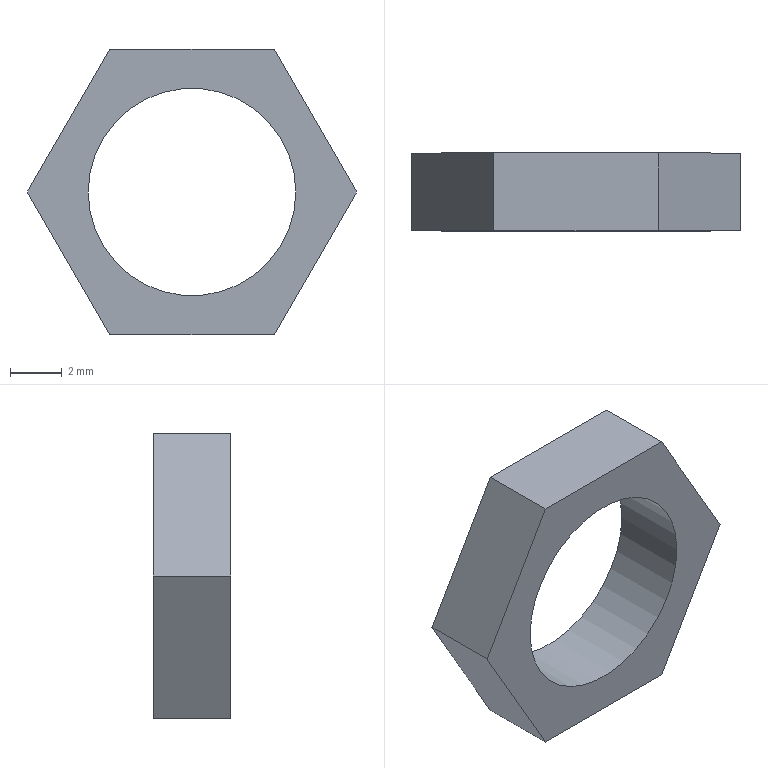Part | STEP file | 1-28.7 | 1 solid | 9 faces | box 12.702 x 3 x 11 mm | volume 163.571 mm3 | plane 8 | cylinder 1 | commonest cylinder face diameters 8 x1
STEP:
#1=CARTESIAN_POINT('',(0.,0.,0.));
#2=DIRECTION('',(0.,0.,1.));
#3=DIRECTION('',(1.,0.,0.));
#4=AXIS2_PLACEMENT_3D('',#1,#2,#3);
#5=CARTESIAN_POINT('',(6.351,0.,0.));
#6=VERTEX_POINT('',#5);
#7=CARTESIAN_POINT('',(3.175,0.,5.5));
#8=VERTEX_POINT('',#7);
#9=CARTESIAN_POINT('',(6.351,0.,0.));
#10=DIRECTION('',(-0.5,0.,0.866));
#11=VECTOR('',#10,1.);
#12=LINE('',#9,#11);
#13=CARTESIAN_POINT('',(0.,0.,0.8509));
#14=DIRECTION('',(0.,-1.,0.));
#15=DIRECTION('',(1.,0.,0.));
#16=AXIS2_PLACEMENT_3D('',#13,#14,#15);
#17=PLANE('',#16);
#18=CARTESIAN_POINT('',(6.351,-0.8509));
#19=DIRECTION('',(-0.5,0.866));
#20=VECTOR('',#19,1.);
#21=LINE('',#18,#20);
#22=(GEOMETRIC_REPRESENTATION_CONTEXT(2)PARAMETRIC_REPRESENTATION_CONTEXT()REPRESENTATION_CONTEXT('',''));
#23=DEFINITIONAL_REPRESENTATION('',(#21),#22);
#24=PCURVE('',#17,#23);
#25=CARTESIAN_POINT('',(4.763,1.5,2.75));
#26=DIRECTION('',(-0.866,0.,-0.5));
#27=DIRECTION('',(-0.5,0.,0.866));
#28=AXIS2_PLACEMENT_3D('',#25,#26,#27);
#29=PLANE('',#28);
#30=CARTESIAN_POINT('',(-3.175,-1.5));
#31=DIRECTION('',(1.,0.));
#32=VECTOR('',#31,1.);
#33=LINE('',#30,#32);
#34=(GEOMETRIC_REPRESENTATION_CONTEXT(2)PARAMETRIC_REPRESENTATION_CONTEXT()REPRESENTATION_CONTEXT('',''));
#35=DEFINITIONAL_REPRESENTATION('',(#33),#34);
#36=PCURVE('',#29,#35);
#37=SURFACE_CURVE('',#12,(#24,#36),.PCURVE_S1.);
#38=EDGE_CURVE('',#6,#8,#37,.T.);
#39=ORIENTED_EDGE('',*,*,#38,.T.);
#40=CARTESIAN_POINT('',(-3.175,0.,5.5));
#41=VERTEX_POINT('',#40);
#42=CARTESIAN_POINT('',(3.175,0.,5.5));
#43=DIRECTION('',(-1.,0.,0.));
#44=VECTOR('',#43,1.);
#45=LINE('',#42,#44);
#46=CARTESIAN_POINT('',(3.175,4.649));
#47=DIRECTION('',(-1.,0.));
#48=VECTOR('',#47,1.);
#49=LINE('',#46,#48);
#50=(GEOMETRIC_REPRESENTATION_CONTEXT(2)PARAMETRIC_REPRESENTATION_CONTEXT()REPRESENTATION_CONTEXT('',''));
#51=DEFINITIONAL_REPRESENTATION('',(#49),#50);
#52=PCURVE('',#17,#51);
#53=CARTESIAN_POINT('',(0.,1.5,5.5));
#54=DIRECTION('',(0.,0.,-1.));
#55=DIRECTION('',(-1.,0.,0.));
#56=AXIS2_PLACEMENT_3D('',#53,#54,#55);
#57=PLANE('',#56);
#58=CARTESIAN_POINT('',(-3.175,-1.5));
#59=DIRECTION('',(1.,0.));
#60=VECTOR('',#59,1.);
#61=LINE('',#58,#60);
#62=(GEOMETRIC_REPRESENTATION_CONTEXT(2)PARAMETRIC_REPRESENTATION_CONTEXT()REPRESENTATION_CONTEXT('',''));
#63=DEFINITIONAL_REPRESENTATION('',(#61),#62);
#64=PCURVE('',#57,#63);
#65=SURFACE_CURVE('',#45,(#52,#64),.PCURVE_S1.);
#66=EDGE_CURVE('',#8,#41,#65,.T.);
#67=ORIENTED_EDGE('',*,*,#66,.T.);
#68=CARTESIAN_POINT('',(-6.351,0.,0.));
#69=VERTEX_POINT('',#68);
#70=CARTESIAN_POINT('',(-3.175,0.,5.5));
#71=DIRECTION('',(-0.5,0.,-0.866));
#72=VECTOR('',#71,1.);
#73=LINE('',#70,#72);
#74=CARTESIAN_POINT('',(-3.175,4.649));
#75=DIRECTION('',(-0.5,-0.866));
#76=VECTOR('',#75,1.);
#77=LINE('',#74,#76);
#78=(GEOMETRIC_REPRESENTATION_CONTEXT(2)PARAMETRIC_REPRESENTATION_CONTEXT()REPRESENTATION_CONTEXT('',''));
#79=DEFINITIONAL_REPRESENTATION('',(#77),#78);
#80=PCURVE('',#17,#79);
#81=CARTESIAN_POINT('',(-4.763,1.5,2.75));
#82=DIRECTION('',(0.866,0.,-0.5));
#83=DIRECTION('',(-0.5,0.,-0.866));
#84=AXIS2_PLACEMENT_3D('',#81,#82,#83);
#85=PLANE('',#84);
#86=CARTESIAN_POINT('',(-3.175,-1.5));
#87=DIRECTION('',(1.,0.));
#88=VECTOR('',#87,1.);
#89=LINE('',#86,#88);
#90=(GEOMETRIC_REPRESENTATION_CONTEXT(2)PARAMETRIC_REPRESENTATION_CONTEXT()REPRESENTATION_CONTEXT('',''));
#91=DEFINITIONAL_REPRESENTATION('',(#89),#90);
#92=PCURVE('',#85,#91);
#93=SURFACE_CURVE('',#73,(#80,#92),.PCURVE_S1.);
#94=EDGE_CURVE('',#41,#69,#93,.T.);
#95=ORIENTED_EDGE('',*,*,#94,.T.);
#96=CARTESIAN_POINT('',(-3.175,0.,-5.5));
#97=VERTEX_POINT('',#96);
#98=CARTESIAN_POINT('',(-6.351,0.,0.));
#99=DIRECTION('',(0.5,0.,-0.866));
#100=VECTOR('',#99,1.);
#101=LINE('',#98,#100);
#102=CARTESIAN_POINT('',(-6.351,-0.8509));
#103=DIRECTION('',(0.5,-0.866));
#104=VECTOR('',#103,1.);
#105=LINE('',#102,#104);
#106=(GEOMETRIC_REPRESENTATION_CONTEXT(2)PARAMETRIC_REPRESENTATION_CONTEXT()REPRESENTATION_CONTEXT('',''));
#107=DEFINITIONAL_REPRESENTATION('',(#105),#106);
#108=PCURVE('',#17,#107);
#109=CARTESIAN_POINT('',(-4.763,1.5,-2.75));
#110=DIRECTION('',(0.866,0.,0.5));
#111=DIRECTION('',(0.5,0.,-0.866));
#112=AXIS2_PLACEMENT_3D('',#109,#110,#111);
#113=PLANE('',#112);
#114=CARTESIAN_POINT('',(-3.175,-1.5));
#115=DIRECTION('',(1.,0.));
#116=VECTOR('',#115,1.);
#117=LINE('',#114,#116);
#118=(GEOMETRIC_REPRESENTATION_CONTEXT(2)PARAMETRIC_REPRESENTATION_CONTEXT()REPRESENTATION_CONTEXT('',''));
#119=DEFINITIONAL_REPRESENTATION('',(#117),#118);
#120=PCURVE('',#113,#119);
#121=SURFACE_CURVE('',#101,(#108,#120),.PCURVE_S1.);
#122=EDGE_CURVE('',#69,#97,#121,.T.);
#123=ORIENTED_EDGE('',*,*,#122,.T.);
#124=CARTESIAN_POINT('',(3.175,0.,-5.5));
#125=VERTEX_POINT('',#124);
#126=CARTESIAN_POINT('',(-3.175,0.,-5.5));
#127=DIRECTION('',(1.,0.,0.));
#128=VECTOR('',#127,1.);
#129=LINE('',#126,#128);
#130=CARTESIAN_POINT('',(-3.175,-6.351));
#131=DIRECTION('',(1.,0.));
#132=VECTOR('',#131,1.);
#133=LINE('',#130,#132);
#134=(GEOMETRIC_REPRESENTATION_CONTEXT(2)PARAMETRIC_REPRESENTATION_CONTEXT()REPRESENTATION_CONTEXT('',''));
#135=DEFINITIONAL_REPRESENTATION('',(#133),#134);
#136=PCURVE('',#17,#135);
#137=CARTESIAN_POINT('',(0.,1.5,-5.5));
#138=DIRECTION('',(0.,0.,1.));
#139=DIRECTION('',(1.,0.,0.));
#140=AXIS2_PLACEMENT_3D('',#137,#138,#139);
#141=PLANE('',#140);
#142=CARTESIAN_POINT('',(-3.175,-1.5));
#143=DIRECTION('',(1.,0.));
#144=VECTOR('',#143,1.);
#145=LINE('',#142,#144);
#146=(GEOMETRIC_REPRESENTATION_CONTEXT(2)PARAMETRIC_REPRESENTATION_CONTEXT()REPRESENTATION_CONTEXT('',''));
#147=DEFINITIONAL_REPRESENTATION('',(#145),#146);
#148=PCURVE('',#141,#147);
#149=SURFACE_CURVE('',#129,(#136,#148),.PCURVE_S1.);
#150=EDGE_CURVE('',#97,#125,#149,.T.);
#151=ORIENTED_EDGE('',*,*,#150,.T.);
#152=CARTESIAN_POINT('',(3.175,0.,-5.5));
#153=DIRECTION('',(0.5,0.,0.866));
#154=VECTOR('',#153,1.);
#155=LINE('',#152,#154);
#156=CARTESIAN_POINT('',(3.175,-6.351));
#157=DIRECTION('',(0.5,0.866));
#158=VECTOR('',#157,1.);
#159=LINE('',#156,#158);
#160=(GEOMETRIC_REPRESENTATION_CONTEXT(2)PARAMETRIC_REPRESENTATION_CONTEXT()REPRESENTATION_CONTEXT('',''));
#161=DEFINITIONAL_REPRESENTATION('',(#159),#160);
#162=PCURVE('',#17,#161);
#163=CARTESIAN_POINT('',(4.763,1.5,-2.75));
#164=DIRECTION('',(-0.866,0.,0.5));
#165=DIRECTION('',(0.5,0.,0.866));
#166=AXIS2_PLACEMENT_3D('',#163,#164,#165);
#167=PLANE('',#166);
#168=CARTESIAN_POINT('',(-3.175,-1.5));
#169=DIRECTION('',(1.,0.));
#170=VECTOR('',#169,1.);
#171=LINE('',#168,#170);
#172=(GEOMETRIC_REPRESENTATION_CONTEXT(2)PARAMETRIC_REPRESENTATION_CONTEXT()REPRESENTATION_CONTEXT('',''));
#173=DEFINITIONAL_REPRESENTATION('',(#171),#172);
#174=PCURVE('',#167,#173);
#175=SURFACE_CURVE('',#155,(#162,#174),.PCURVE_S1.);
#176=EDGE_CURVE('',#125,#6,#175,.T.);
#177=ORIENTED_EDGE('',*,*,#176,.T.);
#178=EDGE_LOOP('',(#39,#67,#95,#123,#151,#177));
#179=FACE_BOUND('',#178,.T.);
#180=CARTESIAN_POINT('',(4.,0.,0.));
#181=VERTEX_POINT('',#180);
#182=CARTESIAN_POINT('',(0.,0.,0.));
#183=DIRECTION('',(0.,1.,0.));
#184=DIRECTION('',(1.,0.,0.));
#185=AXIS2_PLACEMENT_3D('',#182,#183,#184);
#186=CIRCLE('',#185,4.);
#187=CARTESIAN_POINT('',(4.,-0.8509));
#188=CARTESIAN_POINT('',(4.,-7.779));
#189=CARTESIAN_POINT('',(-2.,-4.315));
#190=CARTESIAN_POINT('',(-8.,-0.8509));
#191=CARTESIAN_POINT('',(-2.,2.613));
#192=CARTESIAN_POINT('',(4.,6.077));
#193=CARTESIAN_POINT('',(4.,-0.8509));
#194=(BOUNDED_CURVE()B_SPLINE_CURVE(2,(#187,#188,#189,#190,#191,#192,#193),.UNSPECIFIED.,.T.,.F.)B_SPLINE_CURVE_WITH_KNOTS((1,2,2,2,2,1),(-2.094,0.,2.094,4.189,6.283,8.378),.UNSPECIFIED.)CURVE()GEOMETRIC_REPRESENTATION_ITEM()RATIONAL_B_SPLINE_CURVE((1.,0.5,1.,0.5,1.,0.5,1.))REPRESENTATION_ITEM(''));
#195=(GEOMETRIC_REPRESENTATION_CONTEXT(2)PARAMETRIC_REPRESENTATION_CONTEXT()REPRESENTATION_CONTEXT('',''));
#196=DEFINITIONAL_REPRESENTATION('',(#194),#195);
#197=PCURVE('',#17,#196);
#198=CARTESIAN_POINT('',(0.,0.,0.));
#199=DIRECTION('',(0.,1.,0.));
#200=DIRECTION('',(1.,0.,0.));
#201=AXIS2_PLACEMENT_3D('',#198,#199,#200);
#202=CYLINDRICAL_SURFACE('',#201,4.);
#203=CARTESIAN_POINT('',(0.,0.));
#204=DIRECTION('',(1.,0.));
#205=VECTOR('',#204,1.);
#206=LINE('',#203,#205);
#207=(GEOMETRIC_REPRESENTATION_CONTEXT(2)PARAMETRIC_REPRESENTATION_CONTEXT()REPRESENTATION_CONTEXT('',''));
#208=DEFINITIONAL_REPRESENTATION('',(#206),#207);
#209=PCURVE('',#202,#208);
#210=SURFACE_CURVE('',#186,(#197,#209),.PCURVE_S1.);
#211=EDGE_CURVE('',#181,#181,#210,.T.);
#212=ORIENTED_EDGE('',*,*,#211,.T.);
#213=EDGE_LOOP('',(#212));
#214=FACE_BOUND('',#213,.T.);
#215=ADVANCED_FACE('',(#179,#214),#17,.T.);
#216=CARTESIAN_POINT('',(6.351,3.,0.));
#217=VERTEX_POINT('',#216);
#218=CARTESIAN_POINT('',(3.175,3.,5.5));
#219=VERTEX_POINT('',#218);
#220=CARTESIAN_POINT('',(6.351,3.,0.));
#221=DIRECTION('',(-0.5,0.,0.866));
#222=VECTOR('',#221,1.);
#223=LINE('',#220,#222);
#224=CARTESIAN_POINT('',(0.,3.,0.8509));
#225=DIRECTION('',(0.,-1.,0.));
#226=DIRECTION('',(1.,0.,0.));
#227=AXIS2_PLACEMENT_3D('',#224,#225,#226);
#228=PLANE('',#227);
#229=CARTESIAN_POINT('',(6.351,-0.8509));
#230=DIRECTION('',(-0.5,0.866));
#231=VECTOR('',#230,1.);
#232=LINE('',#229,#231);
#233=(GEOMETRIC_REPRESENTATION_CONTEXT(2)PARAMETRIC_REPRESENTATION_CONTEXT()REPRESENTATION_CONTEXT('',''));
#234=DEFINITIONAL_REPRESENTATION('',(#232),#233);
#235=PCURVE('',#228,#234);
#236=CARTESIAN_POINT('',(-3.175,1.5));
#237=DIRECTION('',(1.,0.));
#238=VECTOR('',#237,1.);
#239=LINE('',#236,#238);
#240=(GEOMETRIC_REPRESENTATION_CONTEXT(2)PARAMETRIC_REPRESENTATION_CONTEXT()REPRESENTATION_CONTEXT('',''));
#241=DEFINITIONAL_REPRESENTATION('',(#239),#240);
#242=PCURVE('',#29,#241);
#243=SURFACE_CURVE('',#223,(#235,#242),.PCURVE_S1.);
#244=EDGE_CURVE('',#217,#219,#243,.T.);
#245=ORIENTED_EDGE('',*,*,#244,.T.);
#246=CARTESIAN_POINT('',(-3.175,3.,5.5));
#247=VERTEX_POINT('',#246);
#248=CARTESIAN_POINT('',(3.175,3.,5.5));
#249=DIRECTION('',(-1.,0.,0.));
#250=VECTOR('',#249,1.);
#251=LINE('',#248,#250);
#252=CARTESIAN_POINT('',(3.175,4.649));
#253=DIRECTION('',(-1.,0.));
#254=VECTOR('',#253,1.);
#255=LINE('',#252,#254);
#256=(GEOMETRIC_REPRESENTATION_CONTEXT(2)PARAMETRIC_REPRESENTATION_CONTEXT()REPRESENTATION_CONTEXT('',''));
#257=DEFINITIONAL_REPRESENTATION('',(#255),#256);
#258=PCURVE('',#228,#257);
#259=CARTESIAN_POINT('',(-3.175,1.5));
#260=DIRECTION('',(1.,0.));
#261=VECTOR('',#260,1.);
#262=LINE('',#259,#261);
#263=(GEOMETRIC_REPRESENTATION_CONTEXT(2)PARAMETRIC_REPRESENTATION_CONTEXT()REPRESENTATION_CONTEXT('',''));
#264=DEFINITIONAL_REPRESENTATION('',(#262),#263);
#265=PCURVE('',#57,#264);
#266=SURFACE_CURVE('',#251,(#258,#265),.PCURVE_S1.);
#267=EDGE_CURVE('',#219,#247,#266,.T.);
#268=ORIENTED_EDGE('',*,*,#267,.T.);
#269=CARTESIAN_POINT('',(-6.351,3.,0.));
#270=VERTEX_POINT('',#269);
#271=CARTESIAN_POINT('',(-3.175,3.,5.5));
#272=DIRECTION('',(-0.5,0.,-0.866));
#273=VECTOR('',#272,1.);
#274=LINE('',#271,#273);
#275=CARTESIAN_POINT('',(-3.175,4.649));
#276=DIRECTION('',(-0.5,-0.866));
#277=VECTOR('',#276,1.);
#278=LINE('',#275,#277);
#279=(GEOMETRIC_REPRESENTATION_CONTEXT(2)PARAMETRIC_REPRESENTATION_CONTEXT()REPRESENTATION_CONTEXT('',''));
#280=DEFINITIONAL_REPRESENTATION('',(#278),#279);
#281=PCURVE('',#228,#280);
#282=CARTESIAN_POINT('',(-3.175,1.5));
#283=DIRECTION('',(1.,0.));
#284=VECTOR('',#283,1.);
#285=LINE('',#282,#284);
#286=(GEOMETRIC_REPRESENTATION_CONTEXT(2)PARAMETRIC_REPRESENTATION_CONTEXT()REPRESENTATION_CONTEXT('',''));
#287=DEFINITIONAL_REPRESENTATION('',(#285),#286);
#288=PCURVE('',#85,#287);
#289=SURFACE_CURVE('',#274,(#281,#288),.PCURVE_S1.);
#290=EDGE_CURVE('',#247,#270,#289,.T.);
#291=ORIENTED_EDGE('',*,*,#290,.T.);
#292=CARTESIAN_POINT('',(-3.175,3.,-5.5));
#293=VERTEX_POINT('',#292);
#294=CARTESIAN_POINT('',(-6.351,3.,0.));
#295=DIRECTION('',(0.5,0.,-0.866));
#296=VECTOR('',#295,1.);
#297=LINE('',#294,#296);
#298=CARTESIAN_POINT('',(-6.351,-0.8509));
#299=DIRECTION('',(0.5,-0.866));
#300=VECTOR('',#299,1.);
#301=LINE('',#298,#300);
#302=(GEOMETRIC_REPRESENTATION_CONTEXT(2)PARAMETRIC_REPRESENTATION_CONTEXT()REPRESENTATION_CONTEXT('',''));
#303=DEFINITIONAL_REPRESENTATION('',(#301),#302);
#304=PCURVE('',#228,#303);
#305=CARTESIAN_POINT('',(-3.175,1.5));
#306=DIRECTION('',(1.,0.));
#307=VECTOR('',#306,1.);
#308=LINE('',#305,#307);
#309=(GEOMETRIC_REPRESENTATION_CONTEXT(2)PARAMETRIC_REPRESENTATION_CONTEXT()REPRESENTATION_CONTEXT('',''));
#310=DEFINITIONAL_REPRESENTATION('',(#308),#309);
#311=PCURVE('',#113,#310);
#312=SURFACE_CURVE('',#297,(#304,#311),.PCURVE_S1.);
#313=EDGE_CURVE('',#270,#293,#312,.T.);
#314=ORIENTED_EDGE('',*,*,#313,.T.);
#315=CARTESIAN_POINT('',(3.175,3.,-5.5));
#316=VERTEX_POINT('',#315);
#317=CARTESIAN_POINT('',(-3.175,3.,-5.5));
#318=DIRECTION('',(1.,0.,0.));
#319=VECTOR('',#318,1.);
#320=LINE('',#317,#319);
#321=CARTESIAN_POINT('',(-3.175,-6.351));
#322=DIRECTION('',(1.,0.));
#323=VECTOR('',#322,1.);
#324=LINE('',#321,#323);
#325=(GEOMETRIC_REPRESENTATION_CONTEXT(2)PARAMETRIC_REPRESENTATION_CONTEXT()REPRESENTATION_CONTEXT('',''));
#326=DEFINITIONAL_REPRESENTATION('',(#324),#325);
#327=PCURVE('',#228,#326);
#328=CARTESIAN_POINT('',(-3.175,1.5));
#329=DIRECTION('',(1.,0.));
#330=VECTOR('',#329,1.);
#331=LINE('',#328,#330);
#332=(GEOMETRIC_REPRESENTATION_CONTEXT(2)PARAMETRIC_REPRESENTATION_CONTEXT()REPRESENTATION_CONTEXT('',''));
#333=DEFINITIONAL_REPRESENTATION('',(#331),#332);
#334=PCURVE('',#141,#333);
#335=SURFACE_CURVE('',#320,(#327,#334),.PCURVE_S1.);
#336=EDGE_CURVE('',#293,#316,#335,.T.);
#337=ORIENTED_EDGE('',*,*,#336,.T.);
#338=CARTESIAN_POINT('',(3.175,3.,-5.5));
#339=DIRECTION('',(0.5,0.,0.866));
#340=VECTOR('',#339,1.);
#341=LINE('',#338,#340);
#342=CARTESIAN_POINT('',(3.175,-6.351));
#343=DIRECTION('',(0.5,0.866));
#344=VECTOR('',#343,1.);
#345=LINE('',#342,#344);
#346=(GEOMETRIC_REPRESENTATION_CONTEXT(2)PARAMETRIC_REPRESENTATION_CONTEXT()REPRESENTATION_CONTEXT('',''));
#347=DEFINITIONAL_REPRESENTATION('',(#345),#346);
#348=PCURVE('',#228,#347);
#349=CARTESIAN_POINT('',(-3.175,1.5));
#350=DIRECTION('',(1.,0.));
#351=VECTOR('',#350,1.);
#352=LINE('',#349,#351);
#353=(GEOMETRIC_REPRESENTATION_CONTEXT(2)PARAMETRIC_REPRESENTATION_CONTEXT()REPRESENTATION_CONTEXT('',''));
#354=DEFINITIONAL_REPRESENTATION('',(#352),#353);
#355=PCURVE('',#167,#354);
#356=SURFACE_CURVE('',#341,(#348,#355),.PCURVE_S1.);
#357=EDGE_CURVE('',#316,#217,#356,.T.);
#358=ORIENTED_EDGE('',*,*,#357,.T.);
#359=EDGE_LOOP('',(#245,#268,#291,#314,#337,#358));
#360=FACE_BOUND('',#359,.F.);
#361=CARTESIAN_POINT('',(4.,3.,0.));
#362=VERTEX_POINT('',#361);
#363=CARTESIAN_POINT('',(0.,3.,0.));
#364=DIRECTION('',(0.,1.,0.));
#365=DIRECTION('',(1.,0.,0.));
#366=AXIS2_PLACEMENT_3D('',#363,#364,#365);
#367=CIRCLE('',#366,4.);
#368=CARTESIAN_POINT('',(4.,-0.8509));
#369=CARTESIAN_POINT('',(4.,-7.779));
#370=CARTESIAN_POINT('',(-2.,-4.315));
#371=CARTESIAN_POINT('',(-8.,-0.8509));
#372=CARTESIAN_POINT('',(-2.,2.613));
#373=CARTESIAN_POINT('',(4.,6.077));
#374=CARTESIAN_POINT('',(4.,-0.8509));
#375=(BOUNDED_CURVE()B_SPLINE_CURVE(2,(#368,#369,#370,#371,#372,#373,#374),.UNSPECIFIED.,.T.,.F.)B_SPLINE_CURVE_WITH_KNOTS((1,2,2,2,2,1),(-2.094,0.,2.094,4.189,6.283,8.378),.UNSPECIFIED.)CURVE()GEOMETRIC_REPRESENTATION_ITEM()RATIONAL_B_SPLINE_CURVE((1.,0.5,1.,0.5,1.,0.5,1.))REPRESENTATION_ITEM(''));
#376=(GEOMETRIC_REPRESENTATION_CONTEXT(2)PARAMETRIC_REPRESENTATION_CONTEXT()REPRESENTATION_CONTEXT('',''));
#377=DEFINITIONAL_REPRESENTATION('',(#375),#376);
#378=PCURVE('',#228,#377);
#379=CARTESIAN_POINT('',(0.,3.));
#380=DIRECTION('',(1.,0.));
#381=VECTOR('',#380,1.);
#382=LINE('',#379,#381);
#383=(GEOMETRIC_REPRESENTATION_CONTEXT(2)PARAMETRIC_REPRESENTATION_CONTEXT()REPRESENTATION_CONTEXT('',''));
#384=DEFINITIONAL_REPRESENTATION('',(#382),#383);
#385=PCURVE('',#202,#384);
#386=SURFACE_CURVE('',#367,(#378,#385),.PCURVE_S1.);
#387=EDGE_CURVE('',#362,#362,#386,.T.);
#388=ORIENTED_EDGE('',*,*,#387,.T.);
#389=EDGE_LOOP('',(#388));
#390=FACE_BOUND('',#389,.F.);
#391=ADVANCED_FACE('',(#360,#390),#228,.F.);
#392=ORIENTED_EDGE('',*,*,#38,.T.);
#393=CARTESIAN_POINT('',(3.175,0.,5.5));
#394=DIRECTION('',(0.,1.,0.));
#395=VECTOR('',#394,1.);
#396=LINE('',#393,#395);
#397=CARTESIAN_POINT('',(3.175,-1.5));
#398=DIRECTION('',(0.,1.));
#399=VECTOR('',#398,1.);
#400=LINE('',#397,#399);
#401=(GEOMETRIC_REPRESENTATION_CONTEXT(2)PARAMETRIC_REPRESENTATION_CONTEXT()REPRESENTATION_CONTEXT('',''));
#402=DEFINITIONAL_REPRESENTATION('',(#400),#401);
#403=PCURVE('',#29,#402);
#404=CARTESIAN_POINT('',(-3.175,-1.5));
#405=DIRECTION('',(0.,1.));
#406=VECTOR('',#405,1.);
#407=LINE('',#404,#406);
#408=(GEOMETRIC_REPRESENTATION_CONTEXT(2)PARAMETRIC_REPRESENTATION_CONTEXT()REPRESENTATION_CONTEXT('',''));
#409=DEFINITIONAL_REPRESENTATION('',(#407),#408);
#410=PCURVE('',#57,#409);
#411=SURFACE_CURVE('',#396,(#403,#410),.PCURVE_S1.);
#412=EDGE_CURVE('',#8,#219,#411,.T.);
#413=ORIENTED_EDGE('',*,*,#412,.T.);
#414=ORIENTED_EDGE('',*,*,#244,.F.);
#415=CARTESIAN_POINT('',(6.351,0.,0.));
#416=DIRECTION('',(0.,1.,0.));
#417=VECTOR('',#416,1.);
#418=LINE('',#415,#417);
#419=CARTESIAN_POINT('',(-3.175,-1.5));
#420=DIRECTION('',(0.,1.));
#421=VECTOR('',#420,1.);
#422=LINE('',#419,#421);
#423=(GEOMETRIC_REPRESENTATION_CONTEXT(2)PARAMETRIC_REPRESENTATION_CONTEXT()REPRESENTATION_CONTEXT('',''));
#424=DEFINITIONAL_REPRESENTATION('',(#422),#423);
#425=PCURVE('',#29,#424);
#426=CARTESIAN_POINT('',(3.175,-1.5));
#427=DIRECTION('',(0.,1.));
#428=VECTOR('',#427,1.);
#429=LINE('',#426,#428);
#430=(GEOMETRIC_REPRESENTATION_CONTEXT(2)PARAMETRIC_REPRESENTATION_CONTEXT()REPRESENTATION_CONTEXT('',''));
#431=DEFINITIONAL_REPRESENTATION('',(#429),#430);
#432=PCURVE('',#167,#431);
#433=SURFACE_CURVE('',#418,(#425,#432),.PCURVE_S1.);
#434=EDGE_CURVE('',#6,#217,#433,.T.);
#435=ORIENTED_EDGE('',*,*,#434,.F.);
#436=EDGE_LOOP('',(#392,#413,#414,#435));
#437=FACE_BOUND('',#436,.F.);
#438=ADVANCED_FACE('',(#437),#29,.F.);
#439=ORIENTED_EDGE('',*,*,#66,.T.);
#440=CARTESIAN_POINT('',(-3.175,0.,5.5));
#441=DIRECTION('',(0.,1.,0.));
#442=VECTOR('',#441,1.);
#443=LINE('',#440,#442);
#444=CARTESIAN_POINT('',(3.175,-1.5));
#445=DIRECTION('',(0.,1.));
#446=VECTOR('',#445,1.);
#447=LINE('',#444,#446);
#448=(GEOMETRIC_REPRESENTATION_CONTEXT(2)PARAMETRIC_REPRESENTATION_CONTEXT()REPRESENTATION_CONTEXT('',''));
#449=DEFINITIONAL_REPRESENTATION('',(#447),#448);
#450=PCURVE('',#57,#449);
#451=CARTESIAN_POINT('',(-3.175,-1.5));
#452=DIRECTION('',(0.,1.));
#453=VECTOR('',#452,1.);
#454=LINE('',#451,#453);
#455=(GEOMETRIC_REPRESENTATION_CONTEXT(2)PARAMETRIC_REPRESENTATION_CONTEXT()REPRESENTATION_CONTEXT('',''));
#456=DEFINITIONAL_REPRESENTATION('',(#454),#455);
#457=PCURVE('',#85,#456);
#458=SURFACE_CURVE('',#443,(#450,#457),.PCURVE_S1.);
#459=EDGE_CURVE('',#41,#247,#458,.T.);
#460=ORIENTED_EDGE('',*,*,#459,.T.);
#461=ORIENTED_EDGE('',*,*,#267,.F.);
#462=ORIENTED_EDGE('',*,*,#412,.F.);
#463=EDGE_LOOP('',(#439,#460,#461,#462));
#464=FACE_BOUND('',#463,.F.);
#465=ADVANCED_FACE('',(#464),#57,.F.);
#466=ORIENTED_EDGE('',*,*,#94,.T.);
#467=CARTESIAN_POINT('',(-6.351,0.,0.));
#468=DIRECTION('',(0.,1.,0.));
#469=VECTOR('',#468,1.);
#470=LINE('',#467,#469);
#471=CARTESIAN_POINT('',(3.175,-1.5));
#472=DIRECTION('',(0.,1.));
#473=VECTOR('',#472,1.);
#474=LINE('',#471,#473);
#475=(GEOMETRIC_REPRESENTATION_CONTEXT(2)PARAMETRIC_REPRESENTATION_CONTEXT()REPRESENTATION_CONTEXT('',''));
#476=DEFINITIONAL_REPRESENTATION('',(#474),#475);
#477=PCURVE('',#85,#476);
#478=CARTESIAN_POINT('',(-3.175,-1.5));
#479=DIRECTION('',(0.,1.));
#480=VECTOR('',#479,1.);
#481=LINE('',#478,#480);
#482=(GEOMETRIC_REPRESENTATION_CONTEXT(2)PARAMETRIC_REPRESENTATION_CONTEXT()REPRESENTATION_CONTEXT('',''));
#483=DEFINITIONAL_REPRESENTATION('',(#481),#482);
#484=PCURVE('',#113,#483);
#485=SURFACE_CURVE('',#470,(#477,#484),.PCURVE_S1.);
#486=EDGE_CURVE('',#69,#270,#485,.T.);
#487=ORIENTED_EDGE('',*,*,#486,.T.);
#488=ORIENTED_EDGE('',*,*,#290,.F.);
#489=ORIENTED_EDGE('',*,*,#459,.F.);
#490=EDGE_LOOP('',(#466,#487,#488,#489));
#491=FACE_BOUND('',#490,.F.);
#492=ADVANCED_FACE('',(#491),#85,.F.);
#493=ORIENTED_EDGE('',*,*,#122,.T.);
#494=CARTESIAN_POINT('',(-3.175,0.,-5.5));
#495=DIRECTION('',(0.,1.,0.));
#496=VECTOR('',#495,1.);
#497=LINE('',#494,#496);
#498=CARTESIAN_POINT('',(3.175,-1.5));
#499=DIRECTION('',(0.,1.));
#500=VECTOR('',#499,1.);
#501=LINE('',#498,#500);
#502=(GEOMETRIC_REPRESENTATION_CONTEXT(2)PARAMETRIC_REPRESENTATION_CONTEXT()REPRESENTATION_CONTEXT('',''));
#503=DEFINITIONAL_REPRESENTATION('',(#501),#502);
#504=PCURVE('',#113,#503);
#505=CARTESIAN_POINT('',(-3.175,-1.5));
#506=DIRECTION('',(0.,1.));
#507=VECTOR('',#506,1.);
#508=LINE('',#505,#507);
#509=(GEOMETRIC_REPRESENTATION_CONTEXT(2)PARAMETRIC_REPRESENTATION_CONTEXT()REPRESENTATION_CONTEXT('',''));
#510=DEFINITIONAL_REPRESENTATION('',(#508),#509);
#511=PCURVE('',#141,#510);
#512=SURFACE_CURVE('',#497,(#504,#511),.PCURVE_S1.);
#513=EDGE_CURVE('',#97,#293,#512,.T.);
#514=ORIENTED_EDGE('',*,*,#513,.T.);
#515=ORIENTED_EDGE('',*,*,#313,.F.);
#516=ORIENTED_EDGE('',*,*,#486,.F.);
#517=EDGE_LOOP('',(#493,#514,#515,#516));
#518=FACE_BOUND('',#517,.F.);
#519=ADVANCED_FACE('',(#518),#113,.F.);
#520=ORIENTED_EDGE('',*,*,#150,.T.);
#521=CARTESIAN_POINT('',(3.175,0.,-5.5));
#522=DIRECTION('',(0.,1.,0.));
#523=VECTOR('',#522,1.);
#524=LINE('',#521,#523);
#525=CARTESIAN_POINT('',(3.175,-1.5));
#526=DIRECTION('',(0.,1.));
#527=VECTOR('',#526,1.);
#528=LINE('',#525,#527);
#529=(GEOMETRIC_REPRESENTATION_CONTEXT(2)PARAMETRIC_REPRESENTATION_CONTEXT()REPRESENTATION_CONTEXT('',''));
#530=DEFINITIONAL_REPRESENTATION('',(#528),#529);
#531=PCURVE('',#141,#530);
#532=CARTESIAN_POINT('',(-3.175,-1.5));
#533=DIRECTION('',(0.,1.));
#534=VECTOR('',#533,1.);
#535=LINE('',#532,#534);
#536=(GEOMETRIC_REPRESENTATION_CONTEXT(2)PARAMETRIC_REPRESENTATION_CONTEXT()REPRESENTATION_CONTEXT('',''));
#537=DEFINITIONAL_REPRESENTATION('',(#535),#536);
#538=PCURVE('',#167,#537);
#539=SURFACE_CURVE('',#524,(#531,#538),.PCURVE_S1.);
#540=EDGE_CURVE('',#125,#316,#539,.T.);
#541=ORIENTED_EDGE('',*,*,#540,.T.);
#542=ORIENTED_EDGE('',*,*,#336,.F.);
#543=ORIENTED_EDGE('',*,*,#513,.F.);
#544=EDGE_LOOP('',(#520,#541,#542,#543));
#545=FACE_BOUND('',#544,.F.);
#546=ADVANCED_FACE('',(#545),#141,.F.);
#547=ORIENTED_EDGE('',*,*,#176,.T.);
#548=ORIENTED_EDGE('',*,*,#434,.T.);
#549=ORIENTED_EDGE('',*,*,#357,.F.);
#550=ORIENTED_EDGE('',*,*,#540,.F.);
#551=EDGE_LOOP('',(#547,#548,#549,#550));
#552=FACE_BOUND('',#551,.F.);
#553=ADVANCED_FACE('',(#552),#167,.F.);
#554=ORIENTED_EDGE('',*,*,#211,.T.);
#555=CARTESIAN_POINT('',(4.,0.,0.));
#556=DIRECTION('',(0.,1.,0.));
#557=VECTOR('',#556,1.);
#558=LINE('',#555,#557);
#559=CARTESIAN_POINT('',(6.283,0.));
#560=DIRECTION('',(0.,1.));
#561=VECTOR('',#560,1.);
#562=LINE('',#559,#561);
#563=(GEOMETRIC_REPRESENTATION_CONTEXT(2)PARAMETRIC_REPRESENTATION_CONTEXT()REPRESENTATION_CONTEXT('',''));
#564=DEFINITIONAL_REPRESENTATION('',(#562),#563);
#565=PCURVE('',#202,#564);
#566=CARTESIAN_POINT('',(0.,0.));
#567=DIRECTION('',(0.,1.));
#568=VECTOR('',#567,1.);
#569=LINE('',#566,#568);
#570=(GEOMETRIC_REPRESENTATION_CONTEXT(2)PARAMETRIC_REPRESENTATION_CONTEXT()REPRESENTATION_CONTEXT('',''));
#571=DEFINITIONAL_REPRESENTATION('',(#569),#570);
#572=PCURVE('',#202,#571);
#573=SEAM_CURVE('',#558,(#565,#572),.PCURVE_S1.);
#574=EDGE_CURVE('',#181,#362,#573,.T.);
#575=ORIENTED_EDGE('',*,*,#574,.T.);
#576=ORIENTED_EDGE('',*,*,#387,.F.);
#577=ORIENTED_EDGE('',*,*,#574,.F.);
#578=EDGE_LOOP('',(#554,#575,#576,#577));
#579=FACE_BOUND('',#578,.F.);
#580=ADVANCED_FACE('',(#579),#202,.F.);
#581=CLOSED_SHELL('',(#215,#391,#438,#465,#492,#519,#546,#553,#580));
#582=MANIFOLD_SOLID_BREP('',#581);
#583=(LENGTH_UNIT()NAMED_UNIT(*)SI_UNIT(.MILLI.,.METRE.));
#584=UNCERTAINTY_MEASURE_WITH_UNIT(LENGTH_MEASURE(0.0000001),#583,'','');
#585=(NAMED_UNIT(*)PLANE_ANGLE_UNIT()SI_UNIT($,.RADIAN.));
#586=(NAMED_UNIT(*)SI_UNIT($,.STERADIAN.)SOLID_ANGLE_UNIT());
#587=(GEOMETRIC_REPRESENTATION_CONTEXT(3)GLOBAL_UNCERTAINTY_ASSIGNED_CONTEXT((#584))GLOBAL_UNIT_ASSIGNED_CONTEXT((#583,#585,#586))REPRESENTATION_CONTEXT('',''));
#588=ADVANCED_BREP_SHAPE_REPRESENTATION('',(#4,#582),#587);